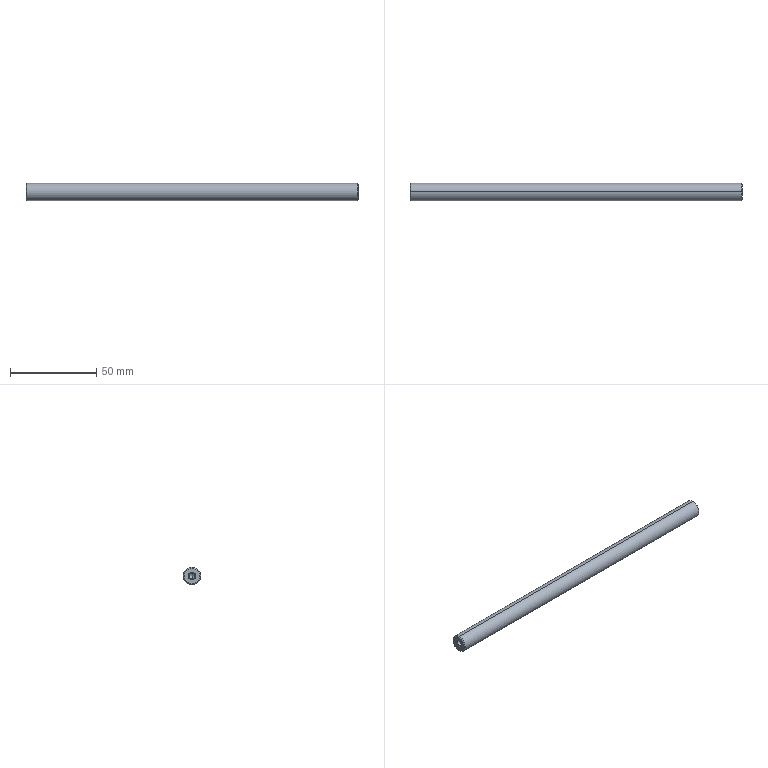Part | STEP file | 04-05 Suction cylinder support rod | 1 solid | 20 faces | box 192 x 10 x 10 mm | volume 14822 mm3 | cone 12 | cylinder 6 | plane 2 | commonest cylinder face diameters 3.3 x4 10 x2